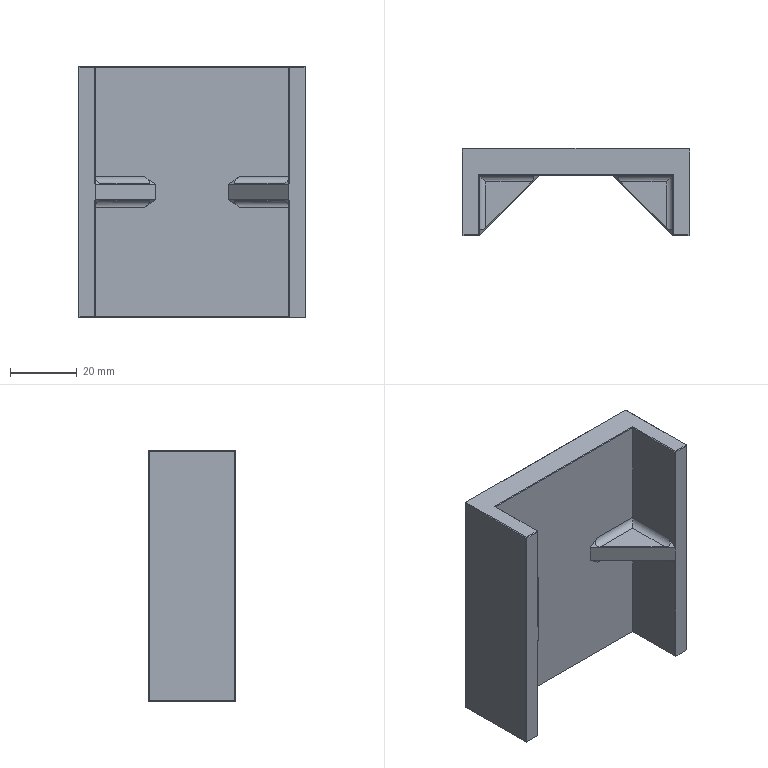Part | STEP file | 2005 | 1 solid | 57 faces | box 68 x 26 x 75 mm | volume 56012 mm3 | plane 49 | cylinder 8 | commonest cylinder face diameters 4 x8